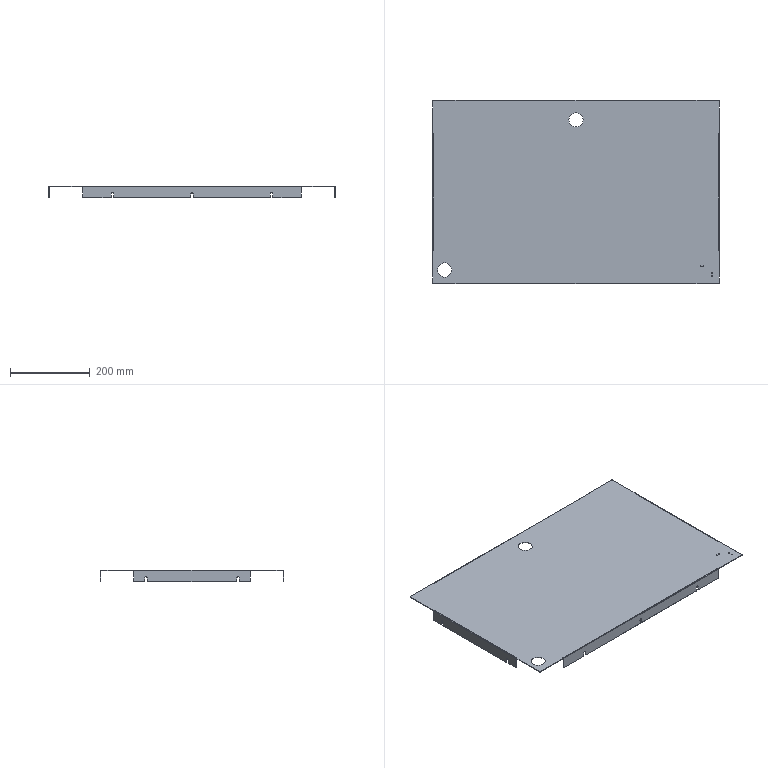Part | STEP file | Lower support plate 1 | 1 solid | 158 faces | box 720 x 462 x 30 mm | volume 565820 mm3 | plane 92 | cylinder 66 | commonest cylinder face diameters 4 x32 6.6 x14 2.5 x8 0.02 x4 3.02 x4 35.5 x4